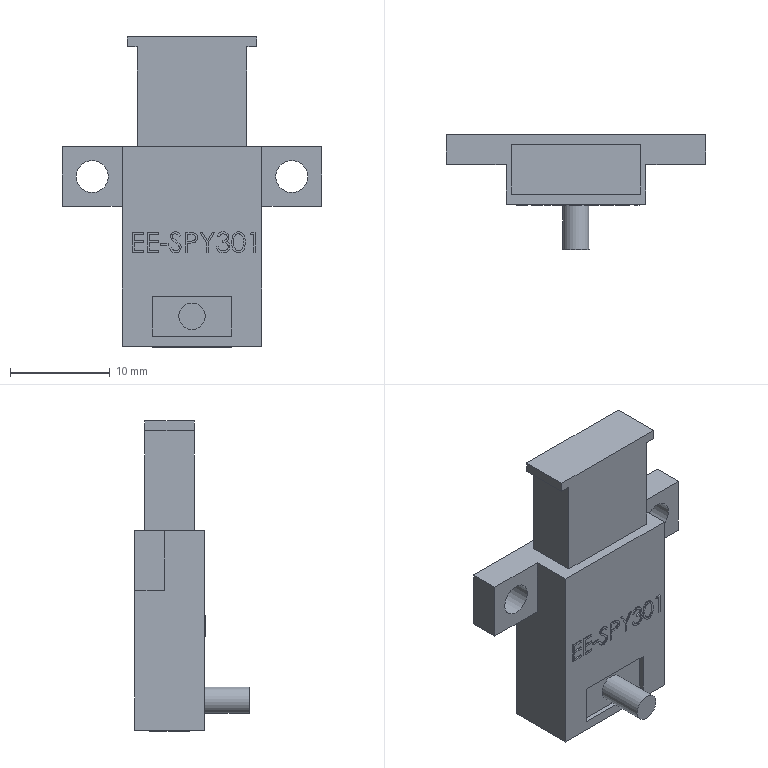Part | NX | 1 solid | 146 faces | box 26 x 11.5 x 31.1 mm | volume 2758 mm3 | plane 99 | spline 44 | cylinder 3 | commonest cylinder face diameters 3.2 x2 2.648 x1